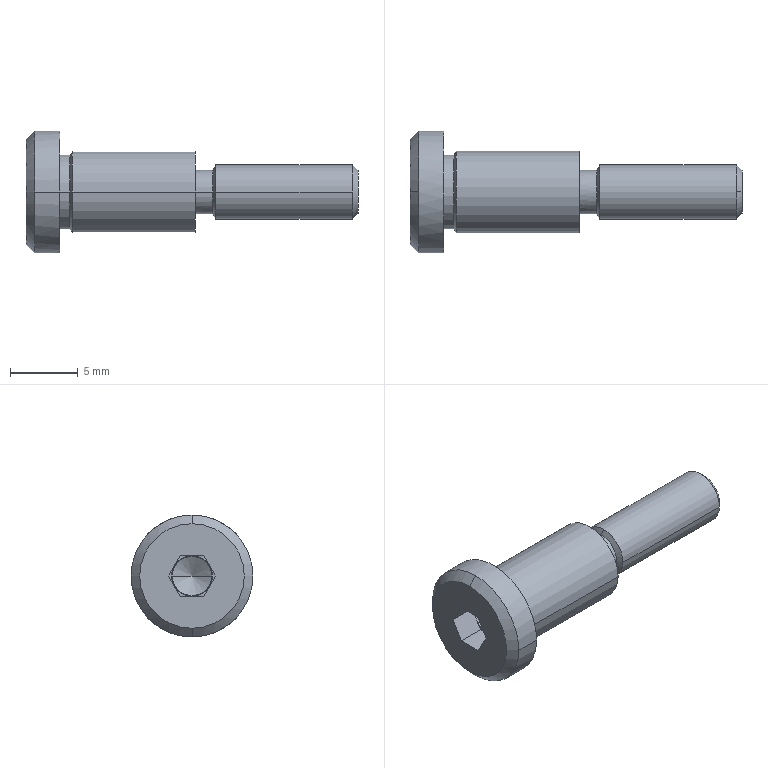Part | SolidWorks | features BaseBody 1 | 1 solid | 40 faces | box 24.5 x 9 x 9 mm | volume 556.102 mm3 | plane 16 | cylinder 12 | cone 10 | spline 2 | commonest cylinder face diameters 3 x2 3.2 x2 4 x2 5.46 x2 6 x2 9 x2
STEP:
#1=CARTESIAN_POINT('',(-0.1825,-1.45,0.));
#2=VERTEX_POINT('',#1);
#3=CARTESIAN_POINT('',(-0.1825,1.45,0.));
#4=VERTEX_POINT('',#3);
#5=CARTESIAN_POINT('',(-0.1825,0.,0.));
#6=DIRECTION('',(-1.,0.,0.));
#7=DIRECTION('',(0.,1.,0.));
#8=AXIS2_PLACEMENT_3D('',#5,#6,#7);
#9=CIRCLE('',#8,1.45);
#10=EDGE_CURVE('',#2,#4,#9,.T.);
#11=ORIENTED_EDGE('',*,*,#10,.F.);
#12=CARTESIAN_POINT('',(-0.2691,-1.5,0.));
#13=VERTEX_POINT('',#12);
#14=CARTESIAN_POINT('',(-0.2691,-1.4,0.));
#15=DIRECTION('',(0.,0.,-1.));
#16=DIRECTION('',(0.,-1.,0.));
#17=AXIS2_PLACEMENT_3D('',#14,#15,#16);
#18=CIRCLE('',#17,0.1);
#19=EDGE_CURVE('',#2,#13,#18,.T.);
#20=ORIENTED_EDGE('',*,*,#19,.T.);
#21=CARTESIAN_POINT('',(-0.2691,1.5,0.));
#22=VERTEX_POINT('',#21);
#23=CARTESIAN_POINT('',(-0.2691,0.,0.));
#24=DIRECTION('',(-1.,0.,0.));
#25=DIRECTION('',(0.,1.,0.));
#26=AXIS2_PLACEMENT_3D('',#23,#24,#25);
#27=CIRCLE('',#26,1.5);
#28=EDGE_CURVE('',#13,#22,#27,.T.);
#29=ORIENTED_EDGE('',*,*,#28,.T.);
#30=CARTESIAN_POINT('',(-0.2691,1.4,0.));
#31=DIRECTION('',(0.,0.,1.));
#32=DIRECTION('',(0.,1.,0.));
#33=AXIS2_PLACEMENT_3D('',#30,#31,#32);
#34=CIRCLE('',#33,0.1);
#35=EDGE_CURVE('',#4,#22,#34,.T.);
#36=ORIENTED_EDGE('',*,*,#35,.F.);
#37=EDGE_LOOP('',(#11,#20,#29,#36));
#38=FACE_OUTER_BOUND('',#37,.T.);
#39=CARTESIAN_POINT('',(-0.1825,1.45,0.));
#40=CARTESIAN_POINT('',(-0.1825,1.45,2.9));
#41=CARTESIAN_POINT('',(-0.1825,-1.45,2.9));
#42=CARTESIAN_POINT('',(-0.1825,-1.45,0.));
#43=CARTESIAN_POINT('',(-0.2008,1.482,0.));
#44=CARTESIAN_POINT('',(-0.2008,1.482,2.963));
#45=CARTESIAN_POINT('',(-0.2008,-1.482,2.963));
#46=CARTESIAN_POINT('',(-0.2008,-1.482,0.));
#47=CARTESIAN_POINT('',(-0.2325,1.5,0.));
#48=CARTESIAN_POINT('',(-0.2325,1.5,3.));
#49=CARTESIAN_POINT('',(-0.2325,-1.5,3.));
#50=CARTESIAN_POINT('',(-0.2325,-1.5,0.));
#51=CARTESIAN_POINT('',(-0.2691,1.5,0.));
#52=CARTESIAN_POINT('',(-0.2691,1.5,3.));
#53=CARTESIAN_POINT('',(-0.2691,-1.5,3.));
#54=CARTESIAN_POINT('',(-0.2691,-1.5,0.));
#55=(BOUNDED_SURFACE()B_SPLINE_SURFACE(3,3,((#39,#40,#41,#42),(#43,#44,#45,#46),(#47,#48,#49,#50),(#51,#52,#53,#54)),.UNSPECIFIED.,.F.,.F.,.F.)B_SPLINE_SURFACE_WITH_KNOTS((4,4),(4,4),(0.,1.),(0.,1.),.UNSPECIFIED.)GEOMETRIC_REPRESENTATION_ITEM()RATIONAL_B_SPLINE_SURFACE(((1.,0.3333,0.3333,1.),(0.9107,0.3036,0.3036,0.9107),(0.9107,0.3036,0.3036,0.9107),(1.,0.3333,0.3333,1.)))REPRESENTATION_ITEM('')SURFACE());
#56=ADVANCED_FACE('',(#38),#55,.F.);
#57=CARTESIAN_POINT('',(0.9,3.,0.));
#58=VERTEX_POINT('',#57);
#59=CARTESIAN_POINT('',(0.9,-3.,0.));
#60=VERTEX_POINT('',#59);
#61=CARTESIAN_POINT('',(0.9,0.,0.));
#62=DIRECTION('',(1.,0.,0.));
#63=DIRECTION('',(0.,1.,0.));
#64=AXIS2_PLACEMENT_3D('',#61,#62,#63);
#65=CIRCLE('',#64,3.);
#66=EDGE_CURVE('',#58,#60,#65,.T.);
#67=ORIENTED_EDGE('',*,*,#66,.T.);
#68=CARTESIAN_POINT('',(10.,-3.,0.));
#69=VERTEX_POINT('',#68);
#70=CARTESIAN_POINT('',(500.,-3.,0.));
#71=DIRECTION('',(1.,0.,0.));
#72=VECTOR('',#71,1000.);
#73=LINE('',#70,#72);
#74=EDGE_CURVE('',#60,#69,#73,.T.);
#75=ORIENTED_EDGE('',*,*,#74,.T.);
#76=CARTESIAN_POINT('',(10.,3.,0.));
#77=VERTEX_POINT('',#76);
#78=CARTESIAN_POINT('',(10.,0.,0.));
#79=DIRECTION('',(-1.,0.,0.));
#80=DIRECTION('',(0.,1.,0.));
#81=AXIS2_PLACEMENT_3D('',#78,#79,#80);
#82=CIRCLE('',#81,3.);
#83=EDGE_CURVE('',#69,#77,#82,.T.);
#84=ORIENTED_EDGE('',*,*,#83,.T.);
#85=CARTESIAN_POINT('',(500.,3.,0.));
#86=DIRECTION('',(1.,0.,0.));
#87=VECTOR('',#86,1000.);
#88=LINE('',#85,#87);
#89=EDGE_CURVE('',#58,#77,#88,.T.);
#90=ORIENTED_EDGE('',*,*,#89,.F.);
#91=EDGE_LOOP('',(#67,#75,#84,#90));
#92=FACE_OUTER_BOUND('',#91,.T.);
#93=CARTESIAN_POINT('',(500.,0.,0.));
#94=DIRECTION('',(1.,0.,0.));
#95=DIRECTION('',(0.,1.,0.));
#96=AXIS2_PLACEMENT_3D('',#93,#94,#95);
#97=CYLINDRICAL_SURFACE('',#96,3.);
#98=ADVANCED_FACE('',(#92),#97,.T.);
#99=CARTESIAN_POINT('',(0.7441,2.73,0.));
#100=VERTEX_POINT('',#99);
#101=CARTESIAN_POINT('',(0.7441,-2.73,0.));
#102=VERTEX_POINT('',#101);
#103=CARTESIAN_POINT('',(0.7441,0.,0.));
#104=DIRECTION('',(1.,0.,0.));
#105=DIRECTION('',(0.,1.,0.));
#106=AXIS2_PLACEMENT_3D('',#103,#104,#105);
#107=CIRCLE('',#106,2.73);
#108=EDGE_CURVE('',#100,#102,#107,.T.);
#109=ORIENTED_EDGE('',*,*,#108,.T.);
#110=CARTESIAN_POINT('',(0.9,-3.,0.));
#111=DIRECTION('',(0.5,-0.866,0.));
#112=VECTOR('',#111,1000.);
#113=LINE('',#110,#112);
#114=EDGE_CURVE('',#102,#60,#113,.T.);
#115=ORIENTED_EDGE('',*,*,#114,.T.);
#116=ORIENTED_EDGE('',*,*,#66,.F.);
#117=CARTESIAN_POINT('',(0.9,3.,0.));
#118=DIRECTION('',(0.5,0.866,0.));
#119=VECTOR('',#118,1000.);
#120=LINE('',#117,#119);
#121=EDGE_CURVE('',#100,#58,#120,.T.);
#122=ORIENTED_EDGE('',*,*,#121,.F.);
#123=EDGE_LOOP('',(#109,#115,#116,#122));
#124=FACE_OUTER_BOUND('',#123,.T.);
#125=CARTESIAN_POINT('',(0.9,0.,0.));
#126=DIRECTION('',(1.,0.,0.));
#127=DIRECTION('',(0.,1.,0.));
#128=AXIS2_PLACEMENT_3D('',#125,#126,#127);
#129=CONICAL_SURFACE('',#128,3.,1.047);
#130=ADVANCED_FACE('',(#124),#129,.T.);
#131=CARTESIAN_POINT('',(0.,2.73,0.));
#132=VERTEX_POINT('',#131);
#133=CARTESIAN_POINT('',(0.,-2.73,0.));
#134=VERTEX_POINT('',#133);
#135=CARTESIAN_POINT('',(0.,0.,0.));
#136=DIRECTION('',(1.,0.,0.));
#137=DIRECTION('',(0.,1.,0.));
#138=AXIS2_PLACEMENT_3D('',#135,#136,#137);
#139=CIRCLE('',#138,2.73);
#140=EDGE_CURVE('',#132,#134,#139,.T.);
#141=ORIENTED_EDGE('',*,*,#140,.T.);
#142=CARTESIAN_POINT('',(500.,-2.73,0.));
#143=DIRECTION('',(1.,0.,0.));
#144=VECTOR('',#143,1000.);
#145=LINE('',#142,#144);
#146=EDGE_CURVE('',#134,#102,#145,.T.);
#147=ORIENTED_EDGE('',*,*,#146,.T.);
#148=ORIENTED_EDGE('',*,*,#108,.F.);
#149=CARTESIAN_POINT('',(500.,2.73,0.));
#150=DIRECTION('',(1.,0.,0.));
#151=VECTOR('',#150,1000.);
#152=LINE('',#149,#151);
#153=EDGE_CURVE('',#132,#100,#152,.T.);
#154=ORIENTED_EDGE('',*,*,#153,.F.);
#155=EDGE_LOOP('',(#141,#147,#148,#154));
#156=FACE_OUTER_BOUND('',#155,.T.);
#157=CARTESIAN_POINT('',(500.,0.,0.));
#158=DIRECTION('',(1.,0.,0.));
#159=DIRECTION('',(0.,1.,0.));
#160=AXIS2_PLACEMENT_3D('',#157,#158,#159);
#161=CYLINDRICAL_SURFACE('',#160,2.73);
#162=ADVANCED_FACE('',(#156),#161,.T.);
#163=CARTESIAN_POINT('',(10.,1.6,0.));
#164=VERTEX_POINT('',#163);
#165=CARTESIAN_POINT('',(10.,-1.6,0.));
#166=VERTEX_POINT('',#165);
#167=CARTESIAN_POINT('',(10.,0.,0.));
#168=DIRECTION('',(1.,0.,0.));
#169=DIRECTION('',(0.,1.,0.));
#170=AXIS2_PLACEMENT_3D('',#167,#168,#169);
#171=CIRCLE('',#170,1.6);
#172=EDGE_CURVE('',#164,#166,#171,.T.);
#173=ORIENTED_EDGE('',*,*,#172,.T.);
#174=CARTESIAN_POINT('',(11.269,-1.6,0.));
#175=VERTEX_POINT('',#174);
#176=CARTESIAN_POINT('',(500.,-1.6,0.));
#177=DIRECTION('',(1.,0.,0.));
#178=VECTOR('',#177,1000.);
#179=LINE('',#176,#178);
#180=EDGE_CURVE('',#166,#175,#179,.T.);
#181=ORIENTED_EDGE('',*,*,#180,.T.);
#182=CARTESIAN_POINT('',(11.269,0.,1.6));
#183=VERTEX_POINT('',#182);
#184=CARTESIAN_POINT('',(11.269,0.,0.));
#185=DIRECTION('',(-1.,0.,0.));
#186=DIRECTION('',(0.,1.,0.));
#187=AXIS2_PLACEMENT_3D('',#184,#185,#186);
#188=CIRCLE('',#187,1.6);
#189=EDGE_CURVE('',#175,#183,#188,.T.);
#190=ORIENTED_EDGE('',*,*,#189,.T.);
#191=CARTESIAN_POINT('',(11.269,1.6,0.));
#192=VERTEX_POINT('',#191);
#193=CARTESIAN_POINT('',(11.269,0.,0.));
#194=DIRECTION('',(-1.,0.,0.));
#195=DIRECTION('',(0.,1.,0.));
#196=AXIS2_PLACEMENT_3D('',#193,#194,#195);
#197=CIRCLE('',#196,1.6);
#198=EDGE_CURVE('',#183,#192,#197,.T.);
#199=ORIENTED_EDGE('',*,*,#198,.T.);
#200=CARTESIAN_POINT('',(500.,1.6,0.));
#201=DIRECTION('',(1.,0.,0.));
#202=VECTOR('',#201,1000.);
#203=LINE('',#200,#202);
#204=EDGE_CURVE('',#164,#192,#203,.T.);
#205=ORIENTED_EDGE('',*,*,#204,.F.);
#206=EDGE_LOOP('',(#173,#181,#190,#199,#205));
#207=FACE_OUTER_BOUND('',#206,.T.);
#208=CARTESIAN_POINT('',(500.,0.,0.));
#209=DIRECTION('',(1.,0.,0.));
#210=DIRECTION('',(0.,1.,0.));
#211=AXIS2_PLACEMENT_3D('',#208,#209,#210);
#212=CYLINDRICAL_SURFACE('',#211,1.6);
#213=ADVANCED_FACE('',(#207),#212,.T.);
#214=ORIENTED_EDGE('',*,*,#198,.F.);
#215=CARTESIAN_POINT('',(11.5,0.,2.));
#216=VERTEX_POINT('',#215);
#217=CARTESIAN_POINT('',(11.5,0.,2.));
#218=DIRECTION('',(0.5,0.,0.866));
#219=VECTOR('',#218,1000.);
#220=LINE('',#217,#219);
#221=EDGE_CURVE('',#183,#216,#220,.T.);
#222=ORIENTED_EDGE('',*,*,#221,.T.);
#223=CARTESIAN_POINT('',(11.5,2.,0.));
#224=VERTEX_POINT('',#223);
#225=CARTESIAN_POINT('',(11.5,0.,0.));
#226=DIRECTION('',(-1.,0.,0.));
#227=DIRECTION('',(0.,1.,0.));
#228=AXIS2_PLACEMENT_3D('',#225,#226,#227);
#229=CIRCLE('',#228,2.);
#230=EDGE_CURVE('',#216,#224,#229,.T.);
#231=ORIENTED_EDGE('',*,*,#230,.T.);
#232=CARTESIAN_POINT('',(11.5,0.,-2.));
#233=VERTEX_POINT('',#232);
#234=CARTESIAN_POINT('',(11.5,0.,0.));
#235=DIRECTION('',(-1.,0.,0.));
#236=DIRECTION('',(0.,1.,0.));
#237=AXIS2_PLACEMENT_3D('',#234,#235,#236);
#238=CIRCLE('',#237,2.);
#239=EDGE_CURVE('',#224,#233,#238,.T.);
#240=ORIENTED_EDGE('',*,*,#239,.T.);
#241=CARTESIAN_POINT('',(11.269,0.,-1.6));
#242=VERTEX_POINT('',#241);
#243=CARTESIAN_POINT('',(11.5,0.,-2.));
#244=DIRECTION('',(0.5,0.,-0.866));
#245=VECTOR('',#244,1000.);
#246=LINE('',#243,#245);
#247=EDGE_CURVE('',#242,#233,#246,.T.);
#248=ORIENTED_EDGE('',*,*,#247,.F.);
#249=CARTESIAN_POINT('',(11.269,0.,0.));
#250=DIRECTION('',(-1.,0.,0.));
#251=DIRECTION('',(0.,1.,0.));
#252=AXIS2_PLACEMENT_3D('',#249,#250,#251);
#253=CIRCLE('',#252,1.6);
#254=EDGE_CURVE('',#192,#242,#253,.T.);
#255=ORIENTED_EDGE('',*,*,#254,.F.);
#256=EDGE_LOOP('',(#214,#222,#231,#240,#248,#255));
#257=FACE_OUTER_BOUND('',#256,.T.);
#258=CARTESIAN_POINT('',(11.5,0.,0.));
#259=DIRECTION('',(1.,0.,0.));
#260=DIRECTION('',(0.,0.,-1.));
#261=AXIS2_PLACEMENT_3D('',#258,#259,#260);
#262=CONICAL_SURFACE('',#261,2.,1.047);
#263=ADVANCED_FACE('',(#257),#262,.T.);
#264=CARTESIAN_POINT('',(-1.864,0.,4.5));
#265=VERTEX_POINT('',#264);
#266=CARTESIAN_POINT('',(-1.864,-4.5,0.));
#267=VERTEX_POINT('',#266);
#268=CARTESIAN_POINT('',(-1.864,0.,0.));
#269=DIRECTION('',(1.,0.,0.));
#270=DIRECTION('',(0.,1.,0.));
#271=AXIS2_PLACEMENT_3D('',#268,#269,#270);
#272=CIRCLE('',#271,4.5);
#273=EDGE_CURVE('',#265,#267,#272,.T.);
#274=ORIENTED_EDGE('',*,*,#273,.T.);
#275=CARTESIAN_POINT('',(0.,-4.5,0.));
#276=VERTEX_POINT('',#275);
#277=CARTESIAN_POINT('',(500.,-4.5,0.));
#278=DIRECTION('',(1.,0.,0.));
#279=VECTOR('',#278,1000.);
#280=LINE('',#277,#279);
#281=EDGE_CURVE('',#267,#276,#280,.T.);
#282=ORIENTED_EDGE('',*,*,#281,.T.);
#283=CARTESIAN_POINT('',(0.,4.5,0.));
#284=VERTEX_POINT('',#283);
#285=CARTESIAN_POINT('',(0.,0.,0.));
#286=DIRECTION('',(-1.,0.,0.));
#287=DIRECTION('',(0.,1.,0.));
#288=AXIS2_PLACEMENT_3D('',#285,#286,#287);
#289=CIRCLE('',#288,4.5);
#290=EDGE_CURVE('',#276,#284,#289,.T.);
#291=ORIENTED_EDGE('',*,*,#290,.T.);
#292=CARTESIAN_POINT('',(-1.864,4.5,0.));
#293=VERTEX_POINT('',#292);
#294=CARTESIAN_POINT('',(500.,4.5,0.));
#295=DIRECTION('',(1.,0.,0.));
#296=VECTOR('',#295,1000.);
#297=LINE('',#294,#296);
#298=EDGE_CURVE('',#293,#284,#297,.T.);
#299=ORIENTED_EDGE('',*,*,#298,.F.);
#300=CARTESIAN_POINT('',(-1.864,0.,0.));
#301=DIRECTION('',(1.,0.,0.));
#302=DIRECTION('',(0.,1.,0.));
#303=AXIS2_PLACEMENT_3D('',#300,#301,#302);
#304=CIRCLE('',#303,4.5);
#305=EDGE_CURVE('',#293,#265,#304,.T.);
#306=ORIENTED_EDGE('',*,*,#305,.T.);
#307=EDGE_LOOP('',(#274,#282,#291,#299,#306));
#308=FACE_OUTER_BOUND('',#307,.T.);
#309=CARTESIAN_POINT('',(500.,0.,0.));
#310=DIRECTION('',(1.,0.,0.));
#311=DIRECTION('',(0.,1.,0.));
#312=AXIS2_PLACEMENT_3D('',#309,#310,#311);
#313=CYLINDRICAL_SURFACE('',#312,4.5);
#314=ADVANCED_FACE('',(#308),#313,.T.);
#315=CARTESIAN_POINT('',(11.5,-2.,0.));
#316=VERTEX_POINT('',#315);
#317=CARTESIAN_POINT('',(11.5,0.,0.));
#318=DIRECTION('',(-1.,0.,0.));
#319=DIRECTION('',(0.,1.,0.));
#320=AXIS2_PLACEMENT_3D('',#317,#318,#319);
#321=CIRCLE('',#320,2.);
#322=EDGE_CURVE('',#316,#216,#321,.T.);
#323=ORIENTED_EDGE('',*,*,#322,.F.);
#324=CARTESIAN_POINT('',(21.57,-2.,0.));
#325=VERTEX_POINT('',#324);
#326=CARTESIAN_POINT('',(500.,-2.,0.));
#327=DIRECTION('',(1.,0.,0.));
#328=VECTOR('',#327,1000.);
#329=LINE('',#326,#328);
#330=EDGE_CURVE('',#316,#325,#329,.T.);
#331=ORIENTED_EDGE('',*,*,#330,.T.);
#332=CARTESIAN_POINT('',(21.57,0.,2.));
#333=VERTEX_POINT('',#332);
#334=CARTESIAN_POINT('',(21.57,0.,0.));
#335=DIRECTION('',(-1.,0.,0.));
#336=DIRECTION('',(0.,1.,0.));
#337=AXIS2_PLACEMENT_3D('',#334,#335,#336);
#338=CIRCLE('',#337,2.);
#339=EDGE_CURVE('',#325,#333,#338,.T.);
#340=ORIENTED_EDGE('',*,*,#339,.T.);
#341=CARTESIAN_POINT('',(21.57,2.,0.));
#342=VERTEX_POINT('',#341);
#343=CARTESIAN_POINT('',(21.57,0.,0.));
#344=DIRECTION('',(-1.,0.,0.));
#345=DIRECTION('',(0.,1.,0.));
#346=AXIS2_PLACEMENT_3D('',#343,#344,#345);
#347=CIRCLE('',#346,2.);
#348=EDGE_CURVE('',#333,#342,#347,.T.);
#349=ORIENTED_EDGE('',*,*,#348,.T.);
#350=CARTESIAN_POINT('',(500.,2.,0.));
#351=DIRECTION('',(1.,0.,0.));
#352=VECTOR('',#351,1000.);
#353=LINE('',#350,#352);
#354=EDGE_CURVE('',#224,#342,#353,.T.);
#355=ORIENTED_EDGE('',*,*,#354,.F.);
#356=ORIENTED_EDGE('',*,*,#230,.F.);
#357=EDGE_LOOP('',(#323,#331,#340,#349,#355,#356));
#358=FACE_OUTER_BOUND('',#357,.T.);
#359=CARTESIAN_POINT('',(500.,0.,0.));
#360=DIRECTION('',(1.,0.,0.));
#361=DIRECTION('',(0.,1.,0.));
#362=AXIS2_PLACEMENT_3D('',#359,#360,#361);
#363=CYLINDRICAL_SURFACE('',#362,2.);
#364=ADVANCED_FACE('',(#358),#363,.T.);
#365=CARTESIAN_POINT('',(-2.5,0.,-3.864));
#366=VERTEX_POINT('',#365);
#367=CARTESIAN_POINT('',(-2.5,0.,3.864));
#368=VERTEX_POINT('',#367);
#369=CARTESIAN_POINT('',(-2.5,0.,0.));
#370=DIRECTION('',(1.,0.,0.));
#371=DIRECTION('',(0.,0.,-1.));
#372=AXIS2_PLACEMENT_3D('',#369,#370,#371);
#373=CIRCLE('',#372,3.864);
#374=EDGE_CURVE('',#366,#368,#373,.T.);
#375=ORIENTED_EDGE('',*,*,#374,.T.);
#376=CARTESIAN_POINT('',(-1.864,0.,4.5));
#377=DIRECTION('',(0.7071,0.,0.7071));
#378=VECTOR('',#377,1000.);
#379=LINE('',#376,#378);
#380=EDGE_CURVE('',#368,#265,#379,.T.);
#381=ORIENTED_EDGE('',*,*,#380,.T.);
#382=ORIENTED_EDGE('',*,*,#305,.F.);
#383=CARTESIAN_POINT('',(-1.864,0.,-4.5));
#384=VERTEX_POINT('',#383);
#385=CARTESIAN_POINT('',(-1.864,0.,0.));
#386=DIRECTION('',(1.,0.,0.));
#387=DIRECTION('',(0.,1.,0.));
#388=AXIS2_PLACEMENT_3D('',#385,#386,#387);
#389=CIRCLE('',#388,4.5);
#390=EDGE_CURVE('',#384,#293,#389,.T.);
#391=ORIENTED_EDGE('',*,*,#390,.F.);
#392=CARTESIAN_POINT('',(-1.864,0.,-4.5));
#393=DIRECTION('',(0.7071,0.,-0.7071));
#394=VECTOR('',#393,1000.);
#395=LINE('',#392,#394);
#396=EDGE_CURVE('',#366,#384,#395,.T.);
#397=ORIENTED_EDGE('',*,*,#396,.F.);
#398=EDGE_LOOP('',(#375,#381,#382,#391,#397));
#399=FACE_OUTER_BOUND('',#398,.T.);
#400=CARTESIAN_POINT('',(-1.864,0.,0.));
#401=DIRECTION('',(1.,0.,0.));
#402=DIRECTION('',(0.,0.,-1.));
#403=AXIS2_PLACEMENT_3D('',#400,#401,#402);
#404=CONICAL_SURFACE('',#403,4.5,0.7854);
#405=ADVANCED_FACE('',(#399),#404,.T.);
#406=CARTESIAN_POINT('',(22.,0.,1.571));
#407=VERTEX_POINT('',#406);
#408=CARTESIAN_POINT('',(22.,0.,-1.571));
#409=VERTEX_POINT('',#408);
#410=CARTESIAN_POINT('',(22.,0.,0.));
#411=DIRECTION('',(-1.,0.,0.));
#412=DIRECTION('',(0.,0.,1.));
#413=AXIS2_PLACEMENT_3D('',#410,#411,#412);
#414=CIRCLE('',#413,1.571);
#415=EDGE_CURVE('',#407,#409,#414,.T.);
#416=ORIENTED_EDGE('',*,*,#415,.T.);
#417=CARTESIAN_POINT('',(21.57,0.,-2.));
#418=VERTEX_POINT('',#417);
#419=CARTESIAN_POINT('',(21.571,0.,-2.));
#420=DIRECTION('',(-0.7071,0.,-0.7071));
#421=VECTOR('',#420,1000.);
#422=LINE('',#419,#421);
#423=EDGE_CURVE('',#409,#418,#422,.T.);
#424=ORIENTED_EDGE('',*,*,#423,.T.);
#425=CARTESIAN_POINT('',(21.57,0.,0.));
#426=DIRECTION('',(-1.,0.,0.));
#427=DIRECTION('',(0.,1.,0.));
#428=AXIS2_PLACEMENT_3D('',#425,#426,#427);
#429=CIRCLE('',#428,2.);
#430=EDGE_CURVE('',#342,#418,#429,.T.);
#431=ORIENTED_EDGE('',*,*,#430,.F.);
#432=ORIENTED_EDGE('',*,*,#348,.F.);
#433=CARTESIAN_POINT('',(21.571,0.,2.));
#434=DIRECTION('',(-0.7071,0.,0.7071));
#435=VECTOR('',#434,1000.);
#436=LINE('',#433,#435);
#437=EDGE_CURVE('',#407,#333,#436,.T.);
#438=ORIENTED_EDGE('',*,*,#437,.F.);
#439=EDGE_LOOP('',(#416,#424,#431,#432,#438));
#440=FACE_OUTER_BOUND('',#439,.T.);
#441=CARTESIAN_POINT('',(21.571,0.,0.));
#442=DIRECTION('',(-1.,0.,0.));
#443=DIRECTION('',(0.,0.,1.));
#444=AXIS2_PLACEMENT_3D('',#441,#442,#443);
#445=CONICAL_SURFACE('',#444,2.,0.7854);
#446=ADVANCED_FACE('',(#440),#445,.T.);
#447=CARTESIAN_POINT('',(-0.5,-1.299,-0.75));
#448=VERTEX_POINT('',#447);
#449=CARTESIAN_POINT('',(-0.5,-1.5,0.));
#450=VERTEX_POINT('',#449);
#451=CARTESIAN_POINT('',(-0.5,0.,0.));
#452=DIRECTION('',(-1.,0.,0.));
#453=DIRECTION('',(0.,1.,0.));
#454=AXIS2_PLACEMENT_3D('',#451,#452,#453);
#455=CIRCLE('',#454,1.5);
#456=EDGE_CURVE('',#448,#450,#455,.T.);
#457=ORIENTED_EDGE('',*,*,#456,.T.);
#458=CARTESIAN_POINT('',(500.,-1.5,0.));
#459=DIRECTION('',(1.,0.,0.));
#460=VECTOR('',#459,1000.);
#461=LINE('',#458,#460);
#462=EDGE_CURVE('',#450,#13,#461,.T.);
#463=ORIENTED_EDGE('',*,*,#462,.T.);
#464=CARTESIAN_POINT('',(-0.2691,0.,0.));
#465=DIRECTION('',(-1.,0.,0.));
#466=DIRECTION('',(0.,1.,0.));
#467=AXIS2_PLACEMENT_3D('',#464,#465,#466);
#468=CIRCLE('',#467,1.5);
#469=EDGE_CURVE('',#22,#13,#468,.T.);
#470=ORIENTED_EDGE('',*,*,#469,.F.);
#471=CARTESIAN_POINT('',(-0.5,1.5,0.));
#472=VERTEX_POINT('',#471);
#473=CARTESIAN_POINT('',(500.,1.5,0.));
#474=DIRECTION('',(1.,0.,0.));
#475=VECTOR('',#474,1000.);
#476=LINE('',#473,#475);
#477=EDGE_CURVE('',#472,#22,#476,.T.);
#478=ORIENTED_EDGE('',*,*,#477,.F.);
#479=CARTESIAN_POINT('',(-0.5,1.299,-0.75));
#480=VERTEX_POINT('',#479);
#481=CARTESIAN_POINT('',(-0.5,0.,0.));
#482=DIRECTION('',(1.,0.,0.));
#483=DIRECTION('',(0.,1.,0.));
#484=AXIS2_PLACEMENT_3D('',#481,#482,#483);
#485=CIRCLE('',#484,1.5);
#486=EDGE_CURVE('',#480,#472,#485,.T.);
#487=ORIENTED_EDGE('',*,*,#486,.F.);
#488=CARTESIAN_POINT('',(-0.5,0.,-1.5));
#489=VERTEX_POINT('',#488);
#490=CARTESIAN_POINT('',(-0.5,0.,0.));
#491=DIRECTION('',(-1.,0.,0.));
#492=DIRECTION('',(0.,1.,0.));
#493=AXIS2_PLACEMENT_3D('',#490,#491,#492);
#494=CIRCLE('',#493,1.5);
#495=EDGE_CURVE('',#480,#489,#494,.T.);
#496=ORIENTED_EDGE('',*,*,#495,.T.);
#497=CARTESIAN_POINT('',(-0.5,0.,0.));
#498=DIRECTION('',(-1.,0.,0.));
#499=DIRECTION('',(0.,1.,0.));
#500=AXIS2_PLACEMENT_3D('',#497,#498,#499);
#501=CIRCLE('',#500,1.5);
#502=EDGE_CURVE('',#489,#448,#501,.T.);
#503=ORIENTED_EDGE('',*,*,#502,.T.);
#504=EDGE_LOOP('',(#457,#463,#470,#478,#487,#496,#503));
#505=FACE_OUTER_BOUND('',#504,.T.);
#506=CARTESIAN_POINT('',(500.,0.,0.));
#507=DIRECTION('',(1.,0.,0.));
#508=DIRECTION('',(0.,1.,0.));
#509=AXIS2_PLACEMENT_3D('',#506,#507,#508);
#510=CYLINDRICAL_SURFACE('',#509,1.5);
#511=ADVANCED_FACE('',(#505),#510,.F.);
#512=CARTESIAN_POINT('',(0.6547,0.,0.));
#513=VERTEX_POINT('',#512);
#514=CARTESIAN_POINT('',(-0.1825,-1.45,0.));
#515=DIRECTION('',(-0.5,-0.866,0.));
#516=VECTOR('',#515,1000.);
#517=LINE('',#514,#516);
#518=EDGE_CURVE('',#513,#2,#517,.T.);
#519=ORIENTED_EDGE('',*,*,#518,.F.);
#520=CARTESIAN_POINT('',(-0.1825,1.45,0.));
#521=DIRECTION('',(-0.5,0.866,0.));
#522=VECTOR('',#521,1000.);
#523=LINE('',#520,#522);
#524=EDGE_CURVE('',#513,#4,#523,.T.);
#525=ORIENTED_EDGE('',*,*,#524,.T.);
#526=CARTESIAN_POINT('',(-0.1825,0.,0.));
#527=DIRECTION('',(-1.,0.,0.));
#528=DIRECTION('',(0.,1.,0.));
#529=AXIS2_PLACEMENT_3D('',#526,#527,#528);
#530=CIRCLE('',#529,1.45);
#531=EDGE_CURVE('',#4,#2,#530,.T.);
#532=ORIENTED_EDGE('',*,*,#531,.T.);
#533=EDGE_LOOP('',(#519,#525,#532));
#534=FACE_OUTER_BOUND('',#533,.T.);
#535=CARTESIAN_POINT('',(-0.1825,0.,0.));
#536=DIRECTION('',(-1.,0.,0.));
#537=DIRECTION('',(0.,-1.,0.));
#538=AXIS2_PLACEMENT_3D('',#535,#536,#537);
#539=CONICAL_SURFACE('',#538,1.45,1.047);
#540=ADVANCED_FACE('',(#534),#539,.F.);
#541=ORIENTED_EDGE('',*,*,#74,.F.);
#542=CARTESIAN_POINT('',(0.9,0.,0.));
#543=DIRECTION('',(1.,0.,0.));
#544=DIRECTION('',(0.,1.,0.));
#545=AXIS2_PLACEMENT_3D('',#542,#543,#544);
#546=CIRCLE('',#545,3.);
#547=EDGE_CURVE('',#60,#58,#546,.T.);
#548=ORIENTED_EDGE('',*,*,#547,.T.);
#549=ORIENTED_EDGE('',*,*,#89,.T.);
#550=CARTESIAN_POINT('',(10.,0.,0.));
#551=DIRECTION('',(-1.,0.,0.));
#552=DIRECTION('',(0.,1.,0.));
#553=AXIS2_PLACEMENT_3D('',#550,#551,#552);
#554=CIRCLE('',#553,3.);
#555=EDGE_CURVE('',#77,#69,#554,.T.);
#556=ORIENTED_EDGE('',*,*,#555,.T.);
#557=EDGE_LOOP('',(#541,#548,#549,#556));
#558=FACE_OUTER_BOUND('',#557,.T.);
#559=CARTESIAN_POINT('',(500.,0.,0.));
#560=DIRECTION('',(1.,0.,0.));
#561=DIRECTION('',(0.,1.,0.));
#562=AXIS2_PLACEMENT_3D('',#559,#560,#561);
#563=CYLINDRICAL_SURFACE('',#562,3.);
#564=ADVANCED_FACE('',(#558),#563,.T.);
#565=ORIENTED_EDGE('',*,*,#114,.F.);
#566=CARTESIAN_POINT('',(0.7441,0.,0.));
#567=DIRECTION('',(1.,0.,0.));
#568=DIRECTION('',(0.,1.,0.));
#569=AXIS2_PLACEMENT_3D('',#566,#567,#568);
#570=CIRCLE('',#569,2.73);
#571=EDGE_CURVE('',#102,#100,#570,.T.);
#572=ORIENTED_EDGE('',*,*,#571,.T.);
#573=ORIENTED_EDGE('',*,*,#121,.T.);
#574=ORIENTED_EDGE('',*,*,#547,.F.);
#575=EDGE_LOOP('',(#565,#572,#573,#574));
#576=FACE_OUTER_BOUND('',#575,.T.);
#577=CARTESIAN_POINT('',(0.9,0.,0.));
#578=DIRECTION('',(1.,0.,0.));
#579=DIRECTION('',(0.,1.,0.));
#580=AXIS2_PLACEMENT_3D('',#577,#578,#579);
#581=CONICAL_SURFACE('',#580,3.,1.047);
#582=ADVANCED_FACE('',(#576),#581,.T.);
#583=ORIENTED_EDGE('',*,*,#555,.F.);
#584=ORIENTED_EDGE('',*,*,#83,.F.);
#585=EDGE_LOOP('',(#583,#584));
#586=FACE_OUTER_BOUND('',#585,.T.);
#587=ORIENTED_EDGE('',*,*,#172,.F.);
#588=CARTESIAN_POINT('',(10.,0.,0.));
#589=DIRECTION('',(1.,0.,0.));
#590=DIRECTION('',(0.,1.,0.));
#591=AXIS2_PLACEMENT_3D('',#588,#589,#590);
#592=CIRCLE('',#591,1.6);
#593=EDGE_CURVE('',#166,#164,#592,.T.);
#594=ORIENTED_EDGE('',*,*,#593,.F.);
#595=EDGE_LOOP('',(#587,#594));
#596=FACE_BOUND('',#595,.T.);
#597=CARTESIAN_POINT('',(10.,3.,0.));
#598=DIRECTION('',(-1.,0.,0.));
#599=DIRECTION('',(0.,-1.,0.));
#600=AXIS2_PLACEMENT_3D('',#597,#598,#599);
#601=PLANE('',#600);
#602=ADVANCED_FACE('',(#586,#596),#601,.F.);
#603=ORIENTED_EDGE('',*,*,#146,.F.);
#604=CARTESIAN_POINT('',(0.,0.,0.));
#605=DIRECTION('',(1.,0.,0.));
#606=DIRECTION('',(0.,1.,0.));
#607=AXIS2_PLACEMENT_3D('',#604,#605,#606);
#608=CIRCLE('',#607,2.73);
#609=EDGE_CURVE('',#134,#132,#608,.T.);
#610=ORIENTED_EDGE('',*,*,#609,.T.);
#611=ORIENTED_EDGE('',*,*,#153,.T.);
#612=ORIENTED_EDGE('',*,*,#571,.F.);
#613=EDGE_LOOP('',(#603,#610,#611,#612));
#614=FACE_OUTER_BOUND('',#613,.T.);
#615=CARTESIAN_POINT('',(500.,0.,0.));
#616=DIRECTION('',(1.,0.,0.));
#617=DIRECTION('',(0.,1.,0.));
#618=AXIS2_PLACEMENT_3D('',#615,#616,#617);
#619=CYLINDRICAL_SURFACE('',#618,2.73);
#620=ADVANCED_FACE('',(#614),#619,.T.);
#621=ORIENTED_EDGE('',*,*,#180,.F.);
#622=ORIENTED_EDGE('',*,*,#593,.T.);
#623=ORIENTED_EDGE('',*,*,#204,.T.);
#624=ORIENTED_EDGE('',*,*,#254,.T.);
#625=CARTESIAN_POINT('',(11.269,0.,0.));
#626=DIRECTION('',(-1.,0.,0.));
#627=DIRECTION('',(0.,1.,0.));
#628=AXIS2_PLACEMENT_3D('',#625,#626,#627);
#629=CIRCLE('',#628,1.6);
#630=EDGE_CURVE('',#242,#175,#629,.T.);
#631=ORIENTED_EDGE('',*,*,#630,.T.);
#632=EDGE_LOOP('',(#621,#622,#623,#624,#631));
#633=FACE_OUTER_BOUND('',#632,.T.);
#634=CARTESIAN_POINT('',(500.,0.,0.));
#635=DIRECTION('',(1.,0.,0.));
#636=DIRECTION('',(0.,1.,0.));
#637=AXIS2_PLACEMENT_3D('',#634,#635,#636);
#638=CYLINDRICAL_SURFACE('',#637,1.6);
#639=ADVANCED_FACE('',(#633),#638,.T.);
#640=CARTESIAN_POINT('',(0.,0.,0.));
#641=DIRECTION('',(-1.,0.,0.));
#642=DIRECTION('',(0.,1.,0.));
#643=AXIS2_PLACEMENT_3D('',#640,#641,#642);
#644=CIRCLE('',#643,4.5);
#645=EDGE_CURVE('',#284,#276,#644,.T.);
#646=ORIENTED_EDGE('',*,*,#645,.F.);
#647=ORIENTED_EDGE('',*,*,#290,.F.);
#648=EDGE_LOOP('',(#646,#647));
#649=FACE_OUTER_BOUND('',#648,.T.);
#650=ORIENTED_EDGE('',*,*,#140,.F.);
#651=ORIENTED_EDGE('',*,*,#609,.F.);
#652=EDGE_LOOP('',(#650,#651));
#653=FACE_BOUND('',#652,.T.);
#654=CARTESIAN_POINT('',(0.,4.5,0.));
#655=DIRECTION('',(-1.,0.,0.));
#656=DIRECTION('',(0.,-1.,0.));
#657=AXIS2_PLACEMENT_3D('',#654,#655,#656);
#658=PLANE('',#657);
#659=ADVANCED_FACE('',(#649,#653),#658,.F.);
#660=ORIENTED_EDGE('',*,*,#221,.F.);
#661=ORIENTED_EDGE('',*,*,#189,.F.);
#662=ORIENTED_EDGE('',*,*,#630,.F.);
#663=ORIENTED_EDGE('',*,*,#247,.T.);
#664=CARTESIAN_POINT('',(11.5,0.,0.));
#665=DIRECTION('',(-1.,0.,0.));
#666=DIRECTION('',(0.,1.,0.));
#667=AXIS2_PLACEMENT_3D('',#664,#665,#666);
#668=CIRCLE('',#667,2.);
#669=EDGE_CURVE('',#233,#316,#668,.T.);
#670=ORIENTED_EDGE('',*,*,#669,.T.);
#671=ORIENTED_EDGE('',*,*,#322,.T.);
#672=EDGE_LOOP('',(#660,#661,#662,#663,#670,#671));
#673=FACE_OUTER_BOUND('',#672,.T.);
#674=CARTESIAN_POINT('',(11.5,0.,0.));
#675=DIRECTION('',(1.,0.,0.));
#676=DIRECTION('',(0.,0.,-1.));
#677=AXIS2_PLACEMENT_3D('',#674,#675,#676);
#678=CONICAL_SURFACE('',#677,2.,1.047);
#679=ADVANCED_FACE('',(#673),#678,.T.);
#680=ORIENTED_EDGE('',*,*,#281,.F.);
#681=CARTESIAN_POINT('',(-1.864,0.,0.));
#682=DIRECTION('',(1.,0.,0.));
#683=DIRECTION('',(0.,1.,0.));
#684=AXIS2_PLACEMENT_3D('',#681,#682,#683);
#685=CIRCLE('',#684,4.5);
#686=EDGE_CURVE('',#267,#384,#685,.T.);
#687=ORIENTED_EDGE('',*,*,#686,.T.);
#688=ORIENTED_EDGE('',*,*,#390,.T.);
#689=ORIENTED_EDGE('',*,*,#298,.T.);
#690=ORIENTED_EDGE('',*,*,#645,.T.);
#691=EDGE_LOOP('',(#680,#687,#688,#689,#690));
#692=FACE_OUTER_BOUND('',#691,.T.);
#693=CARTESIAN_POINT('',(500.,0.,0.));
#694=DIRECTION('',(1.,0.,0.));
#695=DIRECTION('',(0.,1.,0.));
#696=AXIS2_PLACEMENT_3D('',#693,#694,#695);
#697=CYLINDRICAL_SURFACE('',#696,4.5);
#698=ADVANCED_FACE('',(#692),#697,.T.);
#699=ORIENTED_EDGE('',*,*,#330,.F.);
#700=ORIENTED_EDGE('',*,*,#669,.F.);
#701=ORIENTED_EDGE('',*,*,#239,.F.);
#702=ORIENTED_EDGE('',*,*,#354,.T.);
#703=ORIENTED_EDGE('',*,*,#430,.T.);
#704=CARTESIAN_POINT('',(21.57,0.,0.));
#705=DIRECTION('',(-1.,0.,0.));
#706=DIRECTION('',(0.,1.,0.));
#707=AXIS2_PLACEMENT_3D('',#704,#705,#706);
#708=CIRCLE('',#707,2.);
#709=EDGE_CURVE('',#418,#325,#708,.T.);
#710=ORIENTED_EDGE('',*,*,#709,.T.);
#711=EDGE_LOOP('',(#699,#700,#701,#702,#703,#710));
#712=FACE_OUTER_BOUND('',#711,.T.);
#713=CARTESIAN_POINT('',(500.,0.,0.));
#714=DIRECTION('',(1.,0.,0.));
#715=DIRECTION('',(0.,1.,0.));
#716=AXIS2_PLACEMENT_3D('',#713,#714,#715);
#717=CYLINDRICAL_SURFACE('',#716,2.);
#718=ADVANCED_FACE('',(#712),#717,.T.);
#719=ORIENTED_EDGE('',*,*,#380,.F.);
#720=CARTESIAN_POINT('',(-2.5,0.,0.));
#721=DIRECTION('',(1.,0.,0.));
#722=DIRECTION('',(0.,0.,-1.));
#723=AXIS2_PLACEMENT_3D('',#720,#721,#722);
#724=CIRCLE('',#723,3.864);
#725=EDGE_CURVE('',#368,#366,#724,.T.);
#726=ORIENTED_EDGE('',*,*,#725,.T.);
#727=ORIENTED_EDGE('',*,*,#396,.T.);
#728=ORIENTED_EDGE('',*,*,#686,.F.);
#729=ORIENTED_EDGE('',*,*,#273,.F.);
#730=EDGE_LOOP('',(#719,#726,#727,#728,#729));
#731=FACE_OUTER_BOUND('',#730,.T.);
#732=CARTESIAN_POINT('',(-1.864,0.,0.));
#733=DIRECTION('',(1.,0.,0.));
#734=DIRECTION('',(0.,0.,-1.));
#735=AXIS2_PLACEMENT_3D('',#732,#733,#734);
#736=CONICAL_SURFACE('',#735,4.5,0.7854);
#737=ADVANCED_FACE('',(#731),#736,.T.);
#738=ORIENTED_EDGE('',*,*,#423,.F.);
#739=CARTESIAN_POINT('',(22.,0.,0.));
#740=DIRECTION('',(-1.,0.,0.));
#741=DIRECTION('',(0.,0.,1.));
#742=AXIS2_PLACEMENT_3D('',#739,#740,#741);
#743=CIRCLE('',#742,1.571);
#744=EDGE_CURVE('',#409,#407,#743,.T.);
#745=ORIENTED_EDGE('',*,*,#744,.T.);
#746=ORIENTED_EDGE('',*,*,#437,.T.);
#747=ORIENTED_EDGE('',*,*,#339,.F.);
#748=ORIENTED_EDGE('',*,*,#709,.F.);
#749=EDGE_LOOP('',(#738,#745,#746,#747,#748));
#750=FACE_OUTER_BOUND('',#749,.T.);
#751=CARTESIAN_POINT('',(21.571,0.,0.));
#752=DIRECTION('',(-1.,0.,0.));
#753=DIRECTION('',(0.,0.,1.));
#754=AXIS2_PLACEMENT_3D('',#751,#752,#753);
#755=CONICAL_SURFACE('',#754,2.,0.7854);
#756=ADVANCED_FACE('',(#750),#755,.T.);
#757=CARTESIAN_POINT('',(-2.5,0.866,-1.5));
#758=VERTEX_POINT('',#757);
#759=CARTESIAN_POINT('',(-2.5,-0.866,-1.5));
#760=VERTEX_POINT('',#759);
#761=CARTESIAN_POINT('',(-2.5,-0.866,-1.5));
#762=DIRECTION('',(0.,-1.,0.));
#763=VECTOR('',#762,1000.);
#764=LINE('',#761,#763);
#765=EDGE_CURVE('',#758,#760,#764,.T.);
#766=ORIENTED_EDGE('',*,*,#765,.F.);
#767=CARTESIAN_POINT('',(-2.5,1.732,0.));
#768=VERTEX_POINT('',#767);
#769=CARTESIAN_POINT('',(-2.5,0.866,-1.5));
#770=DIRECTION('',(0.,-0.5,-0.866));
#771=VECTOR('',#770,1000.);
#772=LINE('',#769,#771);
#773=EDGE_CURVE('',#768,#758,#772,.T.);
#774=ORIENTED_EDGE('',*,*,#773,.F.);
#775=CARTESIAN_POINT('',(-2.5,0.866,1.5));
#776=VERTEX_POINT('',#775);
#777=CARTESIAN_POINT('',(-2.5,1.732,0.));
#778=DIRECTION('',(0.,0.5,-0.866));
#779=VECTOR('',#778,1000.);
#780=LINE('',#777,#779);
#781=EDGE_CURVE('',#776,#768,#780,.T.);
#782=ORIENTED_EDGE('',*,*,#781,.F.);
#783=CARTESIAN_POINT('',(-2.5,-0.866,1.5));
#784=VERTEX_POINT('',#783);
#785=CARTESIAN_POINT('',(-2.5,0.866,1.5));
#786=DIRECTION('',(0.,1.,0.));
#787=VECTOR('',#786,1000.);
#788=LINE('',#785,#787);
#789=EDGE_CURVE('',#784,#776,#788,.T.);
#790=ORIENTED_EDGE('',*,*,#789,.F.);
#791=CARTESIAN_POINT('',(-2.5,-1.732,0.));
#792=VERTEX_POINT('',#791);
#793=CARTESIAN_POINT('',(-2.5,-0.866,1.5));
#794=DIRECTION('',(0.,0.5,0.866));
#795=VECTOR('',#794,1000.);
#796=LINE('',#793,#795);
#797=EDGE_CURVE('',#792,#784,#796,.T.);
#798=ORIENTED_EDGE('',*,*,#797,.F.);
#799=CARTESIAN_POINT('',(-2.5,-0.866,-1.5));
#800=DIRECTION('',(0.,-0.5,0.866));
#801=VECTOR('',#800,1000.);
#802=LINE('',#799,#801);
#803=EDGE_CURVE('',#760,#792,#802,.T.);
#804=ORIENTED_EDGE('',*,*,#803,.F.);
#805=EDGE_LOOP('',(#766,#774,#782,#790,#798,#804));
#806=FACE_BOUND('',#805,.T.);
#807=ORIENTED_EDGE('',*,*,#374,.F.);
#808=ORIENTED_EDGE('',*,*,#725,.F.);
#809=EDGE_LOOP('',(#807,#808));
#810=FACE_OUTER_BOUND('',#809,.T.);
#811=CARTESIAN_POINT('',(-2.5,1.5,0.));
#812=DIRECTION('',(1.,0.,0.));
#813=DIRECTION('',(0.,1.,0.));
#814=AXIS2_PLACEMENT_3D('',#811,#812,#813);
#815=PLANE('',#814);
#816=ADVANCED_FACE('',(#806,#810),#815,.F.);
#817=ORIENTED_EDGE('',*,*,#415,.F.);
#818=ORIENTED_EDGE('',*,*,#744,.F.);
#819=EDGE_LOOP('',(#817,#818));
#820=FACE_OUTER_BOUND('',#819,.T.);
#821=CARTESIAN_POINT('',(22.,1.571,0.));
#822=DIRECTION('',(-1.,0.,0.));
#823=DIRECTION('',(0.,-1.,0.));
#824=AXIS2_PLACEMENT_3D('',#821,#822,#823);
#825=PLANE('',#824);
#826=ADVANCED_FACE('',(#820),#825,.F.);
#827=ORIENTED_EDGE('',*,*,#803,.T.);
#828=CARTESIAN_POINT('',(-0.5,-1.732,0.));
#829=VERTEX_POINT('',#828);
#830=CARTESIAN_POINT('',(-0.5,-1.732,0.));
#831=DIRECTION('',(1.,0.,0.));
#832=VECTOR('',#831,1000.);
#833=LINE('',#830,#832);
#834=EDGE_CURVE('',#792,#829,#833,.T.);
#835=ORIENTED_EDGE('',*,*,#834,.T.);
#836=CARTESIAN_POINT('',(-0.5,-1.732,0.));
#837=DIRECTION('',(0.,0.5,-0.866));
#838=VECTOR('',#837,1000.);
#839=LINE('',#836,#838);
#840=EDGE_CURVE('',#829,#448,#839,.T.);
#841=ORIENTED_EDGE('',*,*,#840,.T.);
#842=CARTESIAN_POINT('',(-0.5,-0.866,-1.5));
#843=VERTEX_POINT('',#842);
#844=CARTESIAN_POINT('',(-0.5,-1.732,0.));
#845=DIRECTION('',(0.,0.5,-0.866));
#846=VECTOR('',#845,1000.);
#847=LINE('',#844,#846);
#848=EDGE_CURVE('',#448,#843,#847,.T.);
#849=ORIENTED_EDGE('',*,*,#848,.T.);
#850=CARTESIAN_POINT('',(-0.5,-0.866,-1.5));
#851=DIRECTION('',(-1.,0.,0.));
#852=VECTOR('',#851,1000.);
#853=LINE('',#850,#852);
#854=EDGE_CURVE('',#843,#760,#853,.T.);
#855=ORIENTED_EDGE('',*,*,#854,.T.);
#856=EDGE_LOOP('',(#827,#835,#841,#849,#855));
#857=FACE_OUTER_BOUND('',#856,.T.);
#858=CARTESIAN_POINT('',(-0.5,-1.732,0.));
#859=DIRECTION('',(0.,0.866,0.5));
#860=DIRECTION('',(0.,-0.5,0.866));
#861=AXIS2_PLACEMENT_3D('',#858,#859,#860);
#862=PLANE('',#861);
#863=ADVANCED_FACE('',(#857),#862,.T.);
#864=ORIENTED_EDGE('',*,*,#797,.T.);
#865=CARTESIAN_POINT('',(-0.5,-0.866,1.5));
#866=VERTEX_POINT('',#865);
#867=CARTESIAN_POINT('',(-0.5,-0.866,1.5));
#868=DIRECTION('',(1.,0.,0.));
#869=VECTOR('',#868,1000.);
#870=LINE('',#867,#869);
#871=EDGE_CURVE('',#784,#866,#870,.T.);
#872=ORIENTED_EDGE('',*,*,#871,.T.);
#873=CARTESIAN_POINT('',(-0.5,-1.299,0.75));
#874=VERTEX_POINT('',#873);
#875=CARTESIAN_POINT('',(-0.5,-0.866,1.5));
#876=DIRECTION('',(0.,-0.5,-0.866));
#877=VECTOR('',#876,1000.);
#878=LINE('',#875,#877);
#879=EDGE_CURVE('',#866,#874,#878,.T.);
#880=ORIENTED_EDGE('',*,*,#879,.T.);
#881=CARTESIAN_POINT('',(-0.5,-0.866,1.5));
#882=DIRECTION('',(0.,-0.5,-0.866));
#883=VECTOR('',#882,1000.);
#884=LINE('',#881,#883);
#885=EDGE_CURVE('',#874,#829,#884,.T.);
#886=ORIENTED_EDGE('',*,*,#885,.T.);
#887=ORIENTED_EDGE('',*,*,#834,.F.);
#888=EDGE_LOOP('',(#864,#872,#880,#886,#887));
#889=FACE_OUTER_BOUND('',#888,.T.);
#890=CARTESIAN_POINT('',(-0.5,-0.866,1.5));
#891=DIRECTION('',(0.,0.866,-0.5));
#892=DIRECTION('',(0.,0.5,0.866));
#893=AXIS2_PLACEMENT_3D('',#890,#891,#892);
#894=PLANE('',#893);
#895=ADVANCED_FACE('',(#889),#894,.T.);
#896=ORIENTED_EDGE('',*,*,#765,.T.);
#897=ORIENTED_EDGE('',*,*,#854,.F.);
#898=CARTESIAN_POINT('',(-0.5,-0.866,-1.5));
#899=DIRECTION('',(0.,1.,0.));
#900=VECTOR('',#899,1000.);
#901=LINE('',#898,#900);
#902=EDGE_CURVE('',#843,#489,#901,.T.);
#903=ORIENTED_EDGE('',*,*,#902,.T.);
#904=CARTESIAN_POINT('',(-0.5,0.866,-1.5));
#905=VERTEX_POINT('',#904);
#906=CARTESIAN_POINT('',(-0.5,-0.866,-1.5));
#907=DIRECTION('',(0.,1.,0.));
#908=VECTOR('',#907,1000.);
#909=LINE('',#906,#908);
#910=EDGE_CURVE('',#489,#905,#909,.T.);
#911=ORIENTED_EDGE('',*,*,#910,.T.);
#912=CARTESIAN_POINT('',(-0.5,0.866,-1.5));
#913=DIRECTION('',(-1.,0.,0.));
#914=VECTOR('',#913,1000.);
#915=LINE('',#912,#914);
#916=EDGE_CURVE('',#905,#758,#915,.T.);
#917=ORIENTED_EDGE('',*,*,#916,.T.);
#918=EDGE_LOOP('',(#896,#897,#903,#911,#917));
#919=FACE_OUTER_BOUND('',#918,.T.);
#920=CARTESIAN_POINT('',(-0.5,-0.866,-1.5));
#921=DIRECTION('',(0.,0.,1.));
#922=DIRECTION('',(1.,0.,0.));
#923=AXIS2_PLACEMENT_3D('',#920,#921,#922);
#924=PLANE('',#923);
#925=ADVANCED_FACE('',(#919),#924,.T.);
#926=ORIENTED_EDGE('',*,*,#848,.F.);
#927=ORIENTED_EDGE('',*,*,#502,.F.);
#928=ORIENTED_EDGE('',*,*,#902,.F.);
#929=EDGE_LOOP('',(#926,#927,#928));
#930=FACE_OUTER_BOUND('',#929,.T.);
#931=CARTESIAN_POINT('',(-0.5,0.,0.));
#932=DIRECTION('',(1.,0.,0.));
#933=DIRECTION('',(0.,0.,-1.));
#934=AXIS2_PLACEMENT_3D('',#931,#932,#933);
#935=PLANE('',#934);
#936=ADVANCED_FACE('',(#930),#935,.F.);
#937=ORIENTED_EDGE('',*,*,#885,.F.);
#938=CARTESIAN_POINT('',(-0.5,0.,0.));
#939=DIRECTION('',(-1.,0.,0.));
#940=DIRECTION('',(0.,1.,0.));
#941=AXIS2_PLACEMENT_3D('',#938,#939,#940);
#942=CIRCLE('',#941,1.5);
#943=EDGE_CURVE('',#450,#874,#942,.T.);
#944=ORIENTED_EDGE('',*,*,#943,.F.);
#945=ORIENTED_EDGE('',*,*,#456,.F.);
#946=ORIENTED_EDGE('',*,*,#840,.F.);
#947=EDGE_LOOP('',(#937,#944,#945,#946));
#948=FACE_OUTER_BOUND('',#947,.T.);
#949=CARTESIAN_POINT('',(-0.5,0.,0.));
#950=DIRECTION('',(1.,0.,0.));
#951=DIRECTION('',(0.,0.,-1.));
#952=AXIS2_PLACEMENT_3D('',#949,#950,#951);
#953=PLANE('',#952);
#954=ADVANCED_FACE('',(#948),#953,.F.);
#955=ORIENTED_EDGE('',*,*,#789,.T.);
#956=CARTESIAN_POINT('',(-0.5,0.866,1.5));
#957=VERTEX_POINT('',#956);
#958=CARTESIAN_POINT('',(-0.5,0.866,1.5));
#959=DIRECTION('',(1.,0.,0.));
#960=VECTOR('',#959,1000.);
#961=LINE('',#958,#960);
#962=EDGE_CURVE('',#776,#957,#961,.T.);
#963=ORIENTED_EDGE('',*,*,#962,.T.);
#964=CARTESIAN_POINT('',(-0.5,0.,1.5));
#965=VERTEX_POINT('',#964);
#966=CARTESIAN_POINT('',(-0.5,0.866,1.5));
#967=DIRECTION('',(0.,-1.,0.));
#968=VECTOR('',#967,1000.);
#969=LINE('',#966,#968);
#970=EDGE_CURVE('',#957,#965,#969,.T.);
#971=ORIENTED_EDGE('',*,*,#970,.T.);
#972=CARTESIAN_POINT('',(-0.5,0.866,1.5));
#973=DIRECTION('',(0.,-1.,0.));
#974=VECTOR('',#973,1000.);
#975=LINE('',#972,#974);
#976=EDGE_CURVE('',#965,#866,#975,.T.);
#977=ORIENTED_EDGE('',*,*,#976,.T.);
#978=ORIENTED_EDGE('',*,*,#871,.F.);
#979=EDGE_LOOP('',(#955,#963,#971,#977,#978));
#980=FACE_OUTER_BOUND('',#979,.T.);
#981=CARTESIAN_POINT('',(-0.5,0.866,1.5));
#982=DIRECTION('',(0.,0.,-1.));
#983=DIRECTION('',(-1.,0.,0.));
#984=AXIS2_PLACEMENT_3D('',#981,#982,#983);
#985=PLANE('',#984);
#986=ADVANCED_FACE('',(#980),#985,.T.);
#987=ORIENTED_EDGE('',*,*,#976,.F.);
#988=CARTESIAN_POINT('',(-0.5,0.,0.));
#989=DIRECTION('',(-1.,0.,0.));
#990=DIRECTION('',(0.,1.,0.));
#991=AXIS2_PLACEMENT_3D('',#988,#989,#990);
#992=CIRCLE('',#991,1.5);
#993=EDGE_CURVE('',#874,#965,#992,.T.);
#994=ORIENTED_EDGE('',*,*,#993,.F.);
#995=ORIENTED_EDGE('',*,*,#879,.F.);
#996=EDGE_LOOP('',(#987,#994,#995));
#997=FACE_OUTER_BOUND('',#996,.T.);
#998=CARTESIAN_POINT('',(-0.5,0.,0.));
#999=DIRECTION('',(1.,0.,0.));
#1000=DIRECTION('',(0.,0.,-1.));
#1001=AXIS2_PLACEMENT_3D('',#998,#999,#1000);
#1002=PLANE('',#1001);
#1003=ADVANCED_FACE('',(#997),#1002,.F.);
#1004=ORIENTED_EDGE('',*,*,#773,.T.);
#1005=ORIENTED_EDGE('',*,*,#916,.F.);
#1006=CARTESIAN_POINT('',(-0.5,0.866,-1.5));
#1007=DIRECTION('',(0.,0.5,0.866));
#1008=VECTOR('',#1007,1000.);
#1009=LINE('',#1006,#1008);
#1010=EDGE_CURVE('',#905,#480,#1009,.T.);
#1011=ORIENTED_EDGE('',*,*,#1010,.T.);
#1012=CARTESIAN_POINT('',(-0.5,1.732,0.));
#1013=VERTEX_POINT('',#1012);
#1014=CARTESIAN_POINT('',(-0.5,0.866,-1.5));
#1015=DIRECTION('',(0.,0.5,0.866));
#1016=VECTOR('',#1015,1000.);
#1017=LINE('',#1014,#1016);
#1018=EDGE_CURVE('',#480,#1013,#1017,.T.);
#1019=ORIENTED_EDGE('',*,*,#1018,.T.);
#1020=CARTESIAN_POINT('',(-0.5,1.732,0.));
#1021=DIRECTION('',(-1.,0.,0.));
#1022=VECTOR('',#1021,1000.);
#1023=LINE('',#1020,#1022);
#1024=EDGE_CURVE('',#1013,#768,#1023,.T.);
#1025=ORIENTED_EDGE('',*,*,#1024,.T.);
#1026=EDGE_LOOP('',(#1004,#1005,#1011,#1019,#1025));
#1027=FACE_OUTER_BOUND('',#1026,.T.);
#1028=CARTESIAN_POINT('',(-0.5,0.866,-1.5));
#1029=DIRECTION('',(0.,-0.866,0.5));
#1030=DIRECTION('',(0.,-0.5,-0.866));
#1031=AXIS2_PLACEMENT_3D('',#1028,#1029,#1030);
#1032=PLANE('',#1031);
#1033=ADVANCED_FACE('',(#1027),#1032,.T.);
#1034=ORIENTED_EDGE('',*,*,#910,.F.);
#1035=ORIENTED_EDGE('',*,*,#495,.F.);
#1036=ORIENTED_EDGE('',*,*,#1010,.F.);
#1037=EDGE_LOOP('',(#1034,#1035,#1036));
#1038=FACE_OUTER_BOUND('',#1037,.T.);
#1039=CARTESIAN_POINT('',(-0.5,0.,0.));
#1040=DIRECTION('',(1.,0.,0.));
#1041=DIRECTION('',(0.,0.,-1.));
#1042=AXIS2_PLACEMENT_3D('',#1039,#1040,#1041);
#1043=PLANE('',#1042);
#1044=ADVANCED_FACE('',(#1038),#1043,.F.);
#1045=ORIENTED_EDGE('',*,*,#462,.F.);
#1046=ORIENTED_EDGE('',*,*,#943,.T.);
#1047=ORIENTED_EDGE('',*,*,#993,.T.);
#1048=CARTESIAN_POINT('',(-0.5,1.299,0.75));
#1049=VERTEX_POINT('',#1048);
#1050=CARTESIAN_POINT('',(-0.5,0.,0.));
#1051=DIRECTION('',(1.,0.,0.));
#1052=DIRECTION('',(0.,1.,0.));
#1053=AXIS2_PLACEMENT_3D('',#1050,#1051,#1052);
#1054=CIRCLE('',#1053,1.5);
#1055=EDGE_CURVE('',#1049,#965,#1054,.T.);
#1056=ORIENTED_EDGE('',*,*,#1055,.F.);
#1057=CARTESIAN_POINT('',(-0.5,0.,0.));
#1058=DIRECTION('',(1.,0.,0.));
#1059=DIRECTION('',(0.,1.,0.));
#1060=AXIS2_PLACEMENT_3D('',#1057,#1058,#1059);
#1061=CIRCLE('',#1060,1.5);
#1062=EDGE_CURVE('',#472,#1049,#1061,.T.);
#1063=ORIENTED_EDGE('',*,*,#1062,.F.);
#1064=ORIENTED_EDGE('',*,*,#477,.T.);
#1065=ORIENTED_EDGE('',*,*,#28,.F.);
#1066=EDGE_LOOP('',(#1045,#1046,#1047,#1056,#1063,#1064,#1065));
#1067=FACE_OUTER_BOUND('',#1066,.T.);
#1068=CARTESIAN_POINT('',(500.,0.,0.));
#1069=DIRECTION('',(1.,0.,0.));
#1070=DIRECTION('',(0.,1.,0.));
#1071=AXIS2_PLACEMENT_3D('',#1068,#1069,#1070);
#1072=CYLINDRICAL_SURFACE('',#1071,1.5);
#1073=ADVANCED_FACE('',(#1067),#1072,.F.);
#1074=ORIENTED_EDGE('',*,*,#781,.T.);
#1075=ORIENTED_EDGE('',*,*,#1024,.F.);
#1076=CARTESIAN_POINT('',(-0.5,1.732,0.));
#1077=DIRECTION('',(0.,-0.5,0.866));
#1078=VECTOR('',#1077,1000.);
#1079=LINE('',#1076,#1078);
#1080=EDGE_CURVE('',#1013,#1049,#1079,.T.);
#1081=ORIENTED_EDGE('',*,*,#1080,.T.);
#1082=CARTESIAN_POINT('',(-0.5,1.732,0.));
#1083=DIRECTION('',(0.,-0.5,0.866));
#1084=VECTOR('',#1083,1000.);
#1085=LINE('',#1082,#1084);
#1086=EDGE_CURVE('',#1049,#957,#1085,.T.);
#1087=ORIENTED_EDGE('',*,*,#1086,.T.);
#1088=ORIENTED_EDGE('',*,*,#962,.F.);
#1089=EDGE_LOOP('',(#1074,#1075,#1081,#1087,#1088));
#1090=FACE_OUTER_BOUND('',#1089,.T.);
#1091=CARTESIAN_POINT('',(-0.5,1.732,0.));
#1092=DIRECTION('',(0.,-0.866,-0.5));
#1093=DIRECTION('',(0.,0.5,-0.866));
#1094=AXIS2_PLACEMENT_3D('',#1091,#1092,#1093);
#1095=PLANE('',#1094);
#1096=ADVANCED_FACE('',(#1090),#1095,.T.);
#1097=ORIENTED_EDGE('',*,*,#1086,.F.);
#1098=ORIENTED_EDGE('',*,*,#1055,.T.);
#1099=ORIENTED_EDGE('',*,*,#970,.F.);
#1100=EDGE_LOOP('',(#1097,#1098,#1099));
#1101=FACE_OUTER_BOUND('',#1100,.T.);
#1102=CARTESIAN_POINT('',(-0.5,0.,0.));
#1103=DIRECTION('',(1.,0.,0.));
#1104=DIRECTION('',(0.,0.,-1.));
#1105=AXIS2_PLACEMENT_3D('',#1102,#1103,#1104);
#1106=PLANE('',#1105);
#1107=ADVANCED_FACE('',(#1101),#1106,.F.);
#1108=ORIENTED_EDGE('',*,*,#1018,.F.);
#1109=ORIENTED_EDGE('',*,*,#486,.T.);
#1110=ORIENTED_EDGE('',*,*,#1062,.T.);
#1111=ORIENTED_EDGE('',*,*,#1080,.F.);
#1112=EDGE_LOOP('',(#1108,#1109,#1110,#1111));
#1113=FACE_OUTER_BOUND('',#1112,.T.);
#1114=CARTESIAN_POINT('',(-0.5,0.,0.));
#1115=DIRECTION('',(1.,0.,0.));
#1116=DIRECTION('',(0.,0.,-1.));
#1117=AXIS2_PLACEMENT_3D('',#1114,#1115,#1116);
#1118=PLANE('',#1117);
#1119=ADVANCED_FACE('',(#1113),#1118,.F.);
#1120=ORIENTED_EDGE('',*,*,#19,.F.);
#1121=ORIENTED_EDGE('',*,*,#531,.F.);
#1122=ORIENTED_EDGE('',*,*,#35,.T.);
#1123=ORIENTED_EDGE('',*,*,#469,.T.);
#1124=EDGE_LOOP('',(#1120,#1121,#1122,#1123));
#1125=FACE_OUTER_BOUND('',#1124,.T.);
#1126=CARTESIAN_POINT('',(-0.1825,-1.45,0.));
#1127=CARTESIAN_POINT('',(-0.1825,-1.45,-2.9));
#1128=CARTESIAN_POINT('',(-0.1825,1.45,-2.9));
#1129=CARTESIAN_POINT('',(-0.1825,1.45,0.));
#1130=CARTESIAN_POINT('',(-0.2008,-1.482,0.));
#1131=CARTESIAN_POINT('',(-0.2008,-1.482,-2.963));
#1132=CARTESIAN_POINT('',(-0.2008,1.482,-2.963));
#1133=CARTESIAN_POINT('',(-0.2008,1.482,0.));
#1134=CARTESIAN_POINT('',(-0.2325,-1.5,0.));
#1135=CARTESIAN_POINT('',(-0.2325,-1.5,-3.));
#1136=CARTESIAN_POINT('',(-0.2325,1.5,-3.));
#1137=CARTESIAN_POINT('',(-0.2325,1.5,0.));
#1138=CARTESIAN_POINT('',(-0.2691,-1.5,0.));
#1139=CARTESIAN_POINT('',(-0.2691,-1.5,-3.));
#1140=CARTESIAN_POINT('',(-0.2691,1.5,-3.));
#1141=CARTESIAN_POINT('',(-0.2691,1.5,0.));
#1142=(BOUNDED_SURFACE()B_SPLINE_SURFACE(3,3,((#1126,#1127,#1128,#1129),(#1130,#1131,#1132,#1133),(#1134,#1135,#1136,#1137),(#1138,#1139,#1140,#1141)),.UNSPECIFIED.,.F.,.F.,.F.)B_SPLINE_SURFACE_WITH_KNOTS((4,4),(4,4),(0.,1.),(0.,1.),.UNSPECIFIED.)GEOMETRIC_REPRESENTATION_ITEM()RATIONAL_B_SPLINE_SURFACE(((1.,0.3333,0.3333,1.),(0.9107,0.3036,0.3036,0.9107),(0.9107,0.3036,0.3036,0.9107),(1.,0.3333,0.3333,1.)))REPRESENTATION_ITEM('')SURFACE());
#1143=ADVANCED_FACE('',(#1125),#1142,.F.);
#1144=ORIENTED_EDGE('',*,*,#524,.F.);
#1145=ORIENTED_EDGE('',*,*,#518,.T.);
#1146=ORIENTED_EDGE('',*,*,#10,.T.);
#1147=EDGE_LOOP('',(#1144,#1145,#1146));
#1148=FACE_OUTER_BOUND('',#1147,.T.);
#1149=CARTESIAN_POINT('',(-0.1825,0.,0.));
#1150=DIRECTION('',(-1.,0.,0.));
#1151=DIRECTION('',(0.,-1.,0.));
#1152=AXIS2_PLACEMENT_3D('',#1149,#1150,#1151);
#1153=CONICAL_SURFACE('',#1152,1.45,1.047);
#1154=ADVANCED_FACE('',(#1148),#1153,.F.);
#1155=CLOSED_SHELL('',(#56,#98,#130,#162,#213,#263,#314,#364,#405,#446,#511,#540,#564,#582,#602,#620,#639,#659,#679,#698,#718,#737,#756,#816,#826,#863,#895,#925,#936,#954,#986,#1003,#1033,#1044,#1073,#1096,#1107,#1119,#1143,#1154));
#1156=MANIFOLD_SOLID_BREP('',#1155);
#1157=CARTESIAN_POINT('',(0.,0.,0.));
#1158=DIRECTION('',(0.,0.,1.));
#1159=DIRECTION('',(1.,0.,0.));
#1160=AXIS2_PLACEMENT_3D('',#1157,#1158,#1159);
#1161=(LENGTH_UNIT()NAMED_UNIT(*)SI_UNIT(.MILLI.,.METRE.));
#1162=UNCERTAINTY_MEASURE_WITH_UNIT(LENGTH_MEASURE(0.00001),#1161,'','');
#1163=(NAMED_UNIT(*)PLANE_ANGLE_UNIT()SI_UNIT($,.RADIAN.));
#1164=(NAMED_UNIT(*)SI_UNIT($,.STERADIAN.)SOLID_ANGLE_UNIT());
#1165=(GEOMETRIC_REPRESENTATION_CONTEXT(3)GLOBAL_UNCERTAINTY_ASSIGNED_CONTEXT((#1162))GLOBAL_UNIT_ASSIGNED_CONTEXT((#1161,#1163,#1164))REPRESENTATION_CONTEXT('',''));
#1166=ADVANCED_BREP_SHAPE_REPRESENTATION('',(#1156,#1160),#1165);